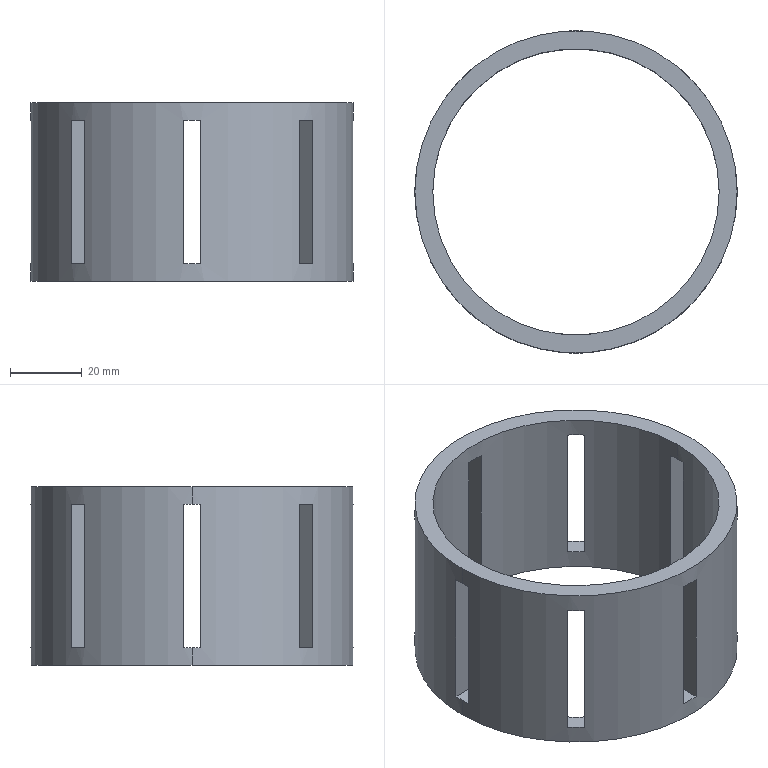Part | SolidWorks | features CirPattern 1, Cut 1, Extrusion 1 | 1 solid | 38 faces | box 90 x 90 x 50 mm | volume 58754 mm3 | plane 34 | cylinder 4 | commonest cylinder face diameters 80 x2 90 x2
STEP:
#1=CARTESIAN_POINT('',(-597.384,-129.922,45.));
#2=VERTEX_POINT('',#1);
#3=CARTESIAN_POINT('',(-597.384,-129.922,5.));
#4=VERTEX_POINT('',#3);
#5=CARTESIAN_POINT('',(-597.384,-129.922,50.));
#6=DIRECTION('',(0.,0.,-1.));
#7=VECTOR('',#6,1000.);
#8=LINE('',#5,#7);
#9=EDGE_CURVE('',#2,#4,#8,.T.);
#10=ORIENTED_EDGE('',*,*,#9,.F.);
#11=CARTESIAN_POINT('',(-602.384,-129.922,45.));
#12=VERTEX_POINT('',#11);
#13=CARTESIAN_POINT('',(-599.884,-90.,45.));
#14=DIRECTION('',(0.,0.,1.));
#15=DIRECTION('',(1.,0.,0.));
#16=AXIS2_PLACEMENT_3D('',#13,#14,#15);
#17=CIRCLE('',#16,40.);
#18=EDGE_CURVE('',#12,#2,#17,.T.);
#19=ORIENTED_EDGE('',*,*,#18,.F.);
#20=CARTESIAN_POINT('',(-602.384,-129.922,5.));
#21=VERTEX_POINT('',#20);
#22=CARTESIAN_POINT('',(-602.384,-129.922,50.));
#23=DIRECTION('',(0.,0.,1.));
#24=VECTOR('',#23,1000.);
#25=LINE('',#22,#24);
#26=EDGE_CURVE('',#21,#12,#25,.T.);
#27=ORIENTED_EDGE('',*,*,#26,.F.);
#28=CARTESIAN_POINT('',(-599.884,-90.,5.));
#29=DIRECTION('',(0.,0.,-1.));
#30=DIRECTION('',(-1.,0.,0.));
#31=AXIS2_PLACEMENT_3D('',#28,#29,#30);
#32=CIRCLE('',#31,40.);
#33=EDGE_CURVE('',#4,#21,#32,.T.);
#34=ORIENTED_EDGE('',*,*,#33,.F.);
#35=EDGE_LOOP('',(#10,#19,#27,#34));
#36=FACE_BOUND('',#35,.T.);
#37=CARTESIAN_POINT('',(-629.881,-116.461,5.));
#38=VERTEX_POINT('',#37);
#39=CARTESIAN_POINT('',(-629.881,-116.461,45.));
#40=VERTEX_POINT('',#39);
#41=CARTESIAN_POINT('',(-629.881,-116.461,50.));
#42=DIRECTION('',(0.,0.,1.));
#43=VECTOR('',#42,1000.);
#44=LINE('',#41,#43);
#45=EDGE_CURVE('',#38,#40,#44,.T.);
#46=ORIENTED_EDGE('',*,*,#45,.F.);
#47=CARTESIAN_POINT('',(-626.345,-119.997,5.));
#48=VERTEX_POINT('',#47);
#49=CARTESIAN_POINT('',(-599.884,-90.,5.));
#50=DIRECTION('',(0.,0.,-1.));
#51=DIRECTION('',(-1.,0.,0.));
#52=AXIS2_PLACEMENT_3D('',#49,#50,#51);
#53=CIRCLE('',#52,40.);
#54=EDGE_CURVE('',#48,#38,#53,.T.);
#55=ORIENTED_EDGE('',*,*,#54,.F.);
#56=CARTESIAN_POINT('',(-626.345,-119.997,45.));
#57=VERTEX_POINT('',#56);
#58=CARTESIAN_POINT('',(-626.345,-119.997,50.));
#59=DIRECTION('',(0.,0.,-1.));
#60=VECTOR('',#59,1000.);
#61=LINE('',#58,#60);
#62=EDGE_CURVE('',#57,#48,#61,.T.);
#63=ORIENTED_EDGE('',*,*,#62,.F.);
#64=CARTESIAN_POINT('',(-599.884,-90.,45.));
#65=DIRECTION('',(0.,0.,1.));
#66=DIRECTION('',(1.,0.,0.));
#67=AXIS2_PLACEMENT_3D('',#64,#65,#66);
#68=CIRCLE('',#67,40.);
#69=EDGE_CURVE('',#40,#57,#68,.T.);
#70=ORIENTED_EDGE('',*,*,#69,.F.);
#71=EDGE_LOOP('',(#46,#55,#63,#70));
#72=FACE_BOUND('',#71,.T.);
#73=CARTESIAN_POINT('',(-569.887,-116.461,45.));
#74=VERTEX_POINT('',#73);
#75=CARTESIAN_POINT('',(-569.887,-116.461,5.));
#76=VERTEX_POINT('',#75);
#77=CARTESIAN_POINT('',(-569.887,-116.461,50.));
#78=DIRECTION('',(0.,0.,-1.));
#79=VECTOR('',#78,1000.);
#80=LINE('',#77,#79);
#81=EDGE_CURVE('',#74,#76,#80,.T.);
#82=ORIENTED_EDGE('',*,*,#81,.F.);
#83=CARTESIAN_POINT('',(-573.423,-119.997,45.));
#84=VERTEX_POINT('',#83);
#85=CARTESIAN_POINT('',(-599.884,-90.,45.));
#86=DIRECTION('',(0.,0.,1.));
#87=DIRECTION('',(1.,0.,0.));
#88=AXIS2_PLACEMENT_3D('',#85,#86,#87);
#89=CIRCLE('',#88,40.);
#90=EDGE_CURVE('',#84,#74,#89,.T.);
#91=ORIENTED_EDGE('',*,*,#90,.F.);
#92=CARTESIAN_POINT('',(-573.423,-119.997,5.));
#93=VERTEX_POINT('',#92);
#94=CARTESIAN_POINT('',(-573.423,-119.997,50.));
#95=DIRECTION('',(0.,0.,1.));
#96=VECTOR('',#95,1000.);
#97=LINE('',#94,#96);
#98=EDGE_CURVE('',#93,#84,#97,.T.);
#99=ORIENTED_EDGE('',*,*,#98,.F.);
#100=CARTESIAN_POINT('',(-599.884,-90.,5.));
#101=DIRECTION('',(0.,0.,-1.));
#102=DIRECTION('',(-1.,0.,0.));
#103=AXIS2_PLACEMENT_3D('',#100,#101,#102);
#104=CIRCLE('',#103,40.);
#105=EDGE_CURVE('',#76,#93,#104,.T.);
#106=ORIENTED_EDGE('',*,*,#105,.F.);
#107=EDGE_LOOP('',(#82,#91,#99,#106));
#108=FACE_BOUND('',#107,.T.);
#109=CARTESIAN_POINT('',(-639.884,-90.,50.));
#110=VERTEX_POINT('',#109);
#111=CARTESIAN_POINT('',(-559.884,-90.,50.));
#112=VERTEX_POINT('',#111);
#113=CARTESIAN_POINT('',(-599.884,-90.,50.));
#114=DIRECTION('',(0.,0.,1.));
#115=DIRECTION('',(1.,0.,0.));
#116=AXIS2_PLACEMENT_3D('',#113,#114,#115);
#117=CIRCLE('',#116,40.);
#118=EDGE_CURVE('',#110,#112,#117,.T.);
#119=ORIENTED_EDGE('',*,*,#118,.T.);
#120=CARTESIAN_POINT('',(-559.884,-90.,45.));
#121=VERTEX_POINT('',#120);
#122=CARTESIAN_POINT('',(-559.884,-90.,50.));
#123=DIRECTION('',(0.,0.,-1.));
#124=VECTOR('',#123,1000.);
#125=LINE('',#122,#124);
#126=EDGE_CURVE('',#112,#121,#125,.T.);
#127=ORIENTED_EDGE('',*,*,#126,.T.);
#128=CARTESIAN_POINT('',(-559.962,-92.5,45.));
#129=VERTEX_POINT('',#128);
#130=CARTESIAN_POINT('',(-599.884,-90.,45.));
#131=DIRECTION('',(0.,0.,1.));
#132=DIRECTION('',(1.,0.,0.));
#133=AXIS2_PLACEMENT_3D('',#130,#131,#132);
#134=CIRCLE('',#133,40.);
#135=EDGE_CURVE('',#129,#121,#134,.T.);
#136=ORIENTED_EDGE('',*,*,#135,.F.);
#137=CARTESIAN_POINT('',(-559.962,-92.5,5.));
#138=VERTEX_POINT('',#137);
#139=CARTESIAN_POINT('',(-559.962,-92.5,50.));
#140=DIRECTION('',(0.,0.,1.));
#141=VECTOR('',#140,1000.);
#142=LINE('',#139,#141);
#143=EDGE_CURVE('',#138,#129,#142,.T.);
#144=ORIENTED_EDGE('',*,*,#143,.F.);
#145=CARTESIAN_POINT('',(-559.884,-90.,5.));
#146=VERTEX_POINT('',#145);
#147=CARTESIAN_POINT('',(-599.884,-90.,5.));
#148=DIRECTION('',(0.,0.,-1.));
#149=DIRECTION('',(-1.,0.,0.));
#150=AXIS2_PLACEMENT_3D('',#147,#148,#149);
#151=CIRCLE('',#150,40.);
#152=EDGE_CURVE('',#146,#138,#151,.T.);
#153=ORIENTED_EDGE('',*,*,#152,.F.);
#154=CARTESIAN_POINT('',(-559.884,-90.,0.));
#155=VERTEX_POINT('',#154);
#156=CARTESIAN_POINT('',(-559.884,-90.,50.));
#157=DIRECTION('',(0.,0.,-1.));
#158=VECTOR('',#157,1000.);
#159=LINE('',#156,#158);
#160=EDGE_CURVE('',#146,#155,#159,.T.);
#161=ORIENTED_EDGE('',*,*,#160,.T.);
#162=CARTESIAN_POINT('',(-639.884,-90.,0.));
#163=VERTEX_POINT('',#162);
#164=CARTESIAN_POINT('',(-599.884,-90.,0.));
#165=DIRECTION('',(0.,0.,1.));
#166=DIRECTION('',(1.,0.,0.));
#167=AXIS2_PLACEMENT_3D('',#164,#165,#166);
#168=CIRCLE('',#167,40.);
#169=EDGE_CURVE('',#163,#155,#168,.T.);
#170=ORIENTED_EDGE('',*,*,#169,.F.);
#171=CARTESIAN_POINT('',(-639.884,-90.,5.));
#172=VERTEX_POINT('',#171);
#173=CARTESIAN_POINT('',(-639.884,-90.,50.));
#174=DIRECTION('',(0.,0.,-1.));
#175=VECTOR('',#174,1000.);
#176=LINE('',#173,#175);
#177=EDGE_CURVE('',#172,#163,#176,.T.);
#178=ORIENTED_EDGE('',*,*,#177,.F.);
#179=CARTESIAN_POINT('',(-639.806,-92.5,5.));
#180=VERTEX_POINT('',#179);
#181=CARTESIAN_POINT('',(-599.884,-90.,5.));
#182=DIRECTION('',(0.,0.,-1.));
#183=DIRECTION('',(-1.,0.,0.));
#184=AXIS2_PLACEMENT_3D('',#181,#182,#183);
#185=CIRCLE('',#184,40.);
#186=EDGE_CURVE('',#180,#172,#185,.T.);
#187=ORIENTED_EDGE('',*,*,#186,.F.);
#188=CARTESIAN_POINT('',(-639.806,-92.5,45.));
#189=VERTEX_POINT('',#188);
#190=CARTESIAN_POINT('',(-639.806,-92.5,50.));
#191=DIRECTION('',(0.,0.,-1.));
#192=VECTOR('',#191,1000.);
#193=LINE('',#190,#192);
#194=EDGE_CURVE('',#189,#180,#193,.T.);
#195=ORIENTED_EDGE('',*,*,#194,.F.);
#196=CARTESIAN_POINT('',(-639.884,-90.,45.));
#197=VERTEX_POINT('',#196);
#198=CARTESIAN_POINT('',(-599.884,-90.,45.));
#199=DIRECTION('',(0.,0.,1.));
#200=DIRECTION('',(1.,0.,0.));
#201=AXIS2_PLACEMENT_3D('',#198,#199,#200);
#202=CIRCLE('',#201,40.);
#203=EDGE_CURVE('',#197,#189,#202,.T.);
#204=ORIENTED_EDGE('',*,*,#203,.F.);
#205=CARTESIAN_POINT('',(-639.884,-90.,50.));
#206=DIRECTION('',(0.,0.,-1.));
#207=VECTOR('',#206,1000.);
#208=LINE('',#205,#207);
#209=EDGE_CURVE('',#110,#197,#208,.T.);
#210=ORIENTED_EDGE('',*,*,#209,.F.);
#211=EDGE_LOOP('',(#119,#127,#136,#144,#153,#161,#170,#178,#187,#195,#204,#210));
#212=FACE_OUTER_BOUND('',#211,.T.);
#213=CARTESIAN_POINT('',(-599.884,-90.,50.));
#214=DIRECTION('',(0.,0.,-1.));
#215=DIRECTION('',(-1.,0.,0.));
#216=AXIS2_PLACEMENT_3D('',#213,#214,#215);
#217=CYLINDRICAL_SURFACE('',#216,40.);
#218=ADVANCED_FACE('',(#36,#72,#108,#212),#217,.F.);
#219=CARTESIAN_POINT('',(-602.384,-45.069,5.));
#220=VERTEX_POINT('',#219);
#221=CARTESIAN_POINT('',(-597.384,-45.069,5.));
#222=VERTEX_POINT('',#221);
#223=CARTESIAN_POINT('',(-599.884,-90.,5.));
#224=DIRECTION('',(0.,0.,-1.));
#225=DIRECTION('',(-1.,0.,0.));
#226=AXIS2_PLACEMENT_3D('',#223,#224,#225);
#227=CIRCLE('',#226,45.);
#228=EDGE_CURVE('',#220,#222,#227,.T.);
#229=ORIENTED_EDGE('',*,*,#228,.T.);
#230=CARTESIAN_POINT('',(-597.384,-45.069,45.));
#231=VERTEX_POINT('',#230);
#232=CARTESIAN_POINT('',(-597.384,-45.069,50.));
#233=DIRECTION('',(0.,0.,1.));
#234=VECTOR('',#233,1000.);
#235=LINE('',#232,#234);
#236=EDGE_CURVE('',#222,#231,#235,.T.);
#237=ORIENTED_EDGE('',*,*,#236,.T.);
#238=CARTESIAN_POINT('',(-602.384,-45.069,45.));
#239=VERTEX_POINT('',#238);
#240=CARTESIAN_POINT('',(-599.884,-90.,45.));
#241=DIRECTION('',(0.,0.,1.));
#242=DIRECTION('',(1.,0.,0.));
#243=AXIS2_PLACEMENT_3D('',#240,#241,#242);
#244=CIRCLE('',#243,45.);
#245=EDGE_CURVE('',#231,#239,#244,.T.);
#246=ORIENTED_EDGE('',*,*,#245,.T.);
#247=CARTESIAN_POINT('',(-602.384,-45.069,50.));
#248=DIRECTION('',(0.,0.,-1.));
#249=VECTOR('',#248,1000.);
#250=LINE('',#247,#249);
#251=EDGE_CURVE('',#239,#220,#250,.T.);
#252=ORIENTED_EDGE('',*,*,#251,.T.);
#253=EDGE_LOOP('',(#229,#237,#246,#252));
#254=FACE_BOUND('',#253,.T.);
#255=CARTESIAN_POINT('',(-566.346,-59.997,45.));
#256=VERTEX_POINT('',#255);
#257=CARTESIAN_POINT('',(-569.881,-56.462,45.));
#258=VERTEX_POINT('',#257);
#259=CARTESIAN_POINT('',(-599.884,-90.,45.));
#260=DIRECTION('',(0.,0.,1.));
#261=DIRECTION('',(1.,0.,0.));
#262=AXIS2_PLACEMENT_3D('',#259,#260,#261);
#263=CIRCLE('',#262,45.);
#264=EDGE_CURVE('',#256,#258,#263,.T.);
#265=ORIENTED_EDGE('',*,*,#264,.T.);
#266=CARTESIAN_POINT('',(-569.881,-56.462,5.));
#267=VERTEX_POINT('',#266);
#268=CARTESIAN_POINT('',(-569.881,-56.462,50.));
#269=DIRECTION('',(0.,0.,-1.));
#270=VECTOR('',#269,1000.);
#271=LINE('',#268,#270);
#272=EDGE_CURVE('',#258,#267,#271,.T.);
#273=ORIENTED_EDGE('',*,*,#272,.T.);
#274=CARTESIAN_POINT('',(-566.346,-59.997,5.));
#275=VERTEX_POINT('',#274);
#276=CARTESIAN_POINT('',(-599.884,-90.,5.));
#277=DIRECTION('',(0.,0.,-1.));
#278=DIRECTION('',(-1.,0.,0.));
#279=AXIS2_PLACEMENT_3D('',#276,#277,#278);
#280=CIRCLE('',#279,45.);
#281=EDGE_CURVE('',#267,#275,#280,.T.);
#282=ORIENTED_EDGE('',*,*,#281,.T.);
#283=CARTESIAN_POINT('',(-566.346,-59.997,50.));
#284=DIRECTION('',(0.,0.,1.));
#285=VECTOR('',#284,1000.);
#286=LINE('',#283,#285);
#287=EDGE_CURVE('',#275,#256,#286,.T.);
#288=ORIENTED_EDGE('',*,*,#287,.T.);
#289=EDGE_LOOP('',(#265,#273,#282,#288));
#290=FACE_BOUND('',#289,.T.);
#291=CARTESIAN_POINT('',(-629.887,-56.462,5.));
#292=VERTEX_POINT('',#291);
#293=CARTESIAN_POINT('',(-629.887,-56.462,45.));
#294=VERTEX_POINT('',#293);
#295=CARTESIAN_POINT('',(-629.887,-56.462,50.));
#296=DIRECTION('',(0.,0.,1.));
#297=VECTOR('',#296,1000.);
#298=LINE('',#295,#297);
#299=EDGE_CURVE('',#292,#294,#298,.T.);
#300=ORIENTED_EDGE('',*,*,#299,.T.);
#301=CARTESIAN_POINT('',(-633.423,-59.997,45.));
#302=VERTEX_POINT('',#301);
#303=CARTESIAN_POINT('',(-599.884,-90.,45.));
#304=DIRECTION('',(0.,0.,1.));
#305=DIRECTION('',(1.,0.,0.));
#306=AXIS2_PLACEMENT_3D('',#303,#304,#305);
#307=CIRCLE('',#306,45.);
#308=EDGE_CURVE('',#294,#302,#307,.T.);
#309=ORIENTED_EDGE('',*,*,#308,.T.);
#310=CARTESIAN_POINT('',(-633.423,-59.997,5.));
#311=VERTEX_POINT('',#310);
#312=CARTESIAN_POINT('',(-633.423,-59.997,50.));
#313=DIRECTION('',(0.,0.,-1.));
#314=VECTOR('',#313,1000.);
#315=LINE('',#312,#314);
#316=EDGE_CURVE('',#302,#311,#315,.T.);
#317=ORIENTED_EDGE('',*,*,#316,.T.);
#318=CARTESIAN_POINT('',(-599.884,-90.,5.));
#319=DIRECTION('',(0.,0.,-1.));
#320=DIRECTION('',(-1.,0.,0.));
#321=AXIS2_PLACEMENT_3D('',#318,#319,#320);
#322=CIRCLE('',#321,45.);
#323=EDGE_CURVE('',#311,#292,#322,.T.);
#324=ORIENTED_EDGE('',*,*,#323,.T.);
#325=EDGE_LOOP('',(#300,#309,#317,#324));
#326=FACE_BOUND('',#325,.T.);
#327=CARTESIAN_POINT('',(-554.884,-90.,50.));
#328=VERTEX_POINT('',#327);
#329=CARTESIAN_POINT('',(-644.884,-90.,50.));
#330=VERTEX_POINT('',#329);
#331=CARTESIAN_POINT('',(-599.884,-90.,50.));
#332=DIRECTION('',(0.,0.,1.));
#333=DIRECTION('',(1.,0.,0.));
#334=AXIS2_PLACEMENT_3D('',#331,#332,#333);
#335=CIRCLE('',#334,45.);
#336=EDGE_CURVE('',#328,#330,#335,.T.);
#337=ORIENTED_EDGE('',*,*,#336,.F.);
#338=CARTESIAN_POINT('',(-554.884,-90.,45.));
#339=VERTEX_POINT('',#338);
#340=CARTESIAN_POINT('',(-554.884,-90.,50.));
#341=DIRECTION('',(0.,0.,-1.));
#342=VECTOR('',#341,1000.);
#343=LINE('',#340,#342);
#344=EDGE_CURVE('',#328,#339,#343,.T.);
#345=ORIENTED_EDGE('',*,*,#344,.T.);
#346=CARTESIAN_POINT('',(-554.954,-87.5,45.));
#347=VERTEX_POINT('',#346);
#348=CARTESIAN_POINT('',(-599.884,-90.,45.));
#349=DIRECTION('',(0.,0.,1.));
#350=DIRECTION('',(1.,0.,0.));
#351=AXIS2_PLACEMENT_3D('',#348,#349,#350);
#352=CIRCLE('',#351,45.);
#353=EDGE_CURVE('',#339,#347,#352,.T.);
#354=ORIENTED_EDGE('',*,*,#353,.T.);
#355=CARTESIAN_POINT('',(-554.954,-87.5,5.));
#356=VERTEX_POINT('',#355);
#357=CARTESIAN_POINT('',(-554.954,-87.5,50.));
#358=DIRECTION('',(0.,0.,-1.));
#359=VECTOR('',#358,1000.);
#360=LINE('',#357,#359);
#361=EDGE_CURVE('',#347,#356,#360,.T.);
#362=ORIENTED_EDGE('',*,*,#361,.T.);
#363=CARTESIAN_POINT('',(-554.884,-90.,5.));
#364=VERTEX_POINT('',#363);
#365=CARTESIAN_POINT('',(-599.884,-90.,5.));
#366=DIRECTION('',(0.,0.,-1.));
#367=DIRECTION('',(-1.,0.,0.));
#368=AXIS2_PLACEMENT_3D('',#365,#366,#367);
#369=CIRCLE('',#368,45.);
#370=EDGE_CURVE('',#356,#364,#369,.T.);
#371=ORIENTED_EDGE('',*,*,#370,.T.);
#372=CARTESIAN_POINT('',(-554.884,-90.,0.));
#373=VERTEX_POINT('',#372);
#374=CARTESIAN_POINT('',(-554.884,-90.,50.));
#375=DIRECTION('',(0.,0.,-1.));
#376=VECTOR('',#375,1000.);
#377=LINE('',#374,#376);
#378=EDGE_CURVE('',#364,#373,#377,.T.);
#379=ORIENTED_EDGE('',*,*,#378,.T.);
#380=CARTESIAN_POINT('',(-644.884,-90.,0.));
#381=VERTEX_POINT('',#380);
#382=CARTESIAN_POINT('',(-599.884,-90.,0.));
#383=DIRECTION('',(0.,0.,1.));
#384=DIRECTION('',(1.,0.,0.));
#385=AXIS2_PLACEMENT_3D('',#382,#383,#384);
#386=CIRCLE('',#385,45.);
#387=EDGE_CURVE('',#373,#381,#386,.T.);
#388=ORIENTED_EDGE('',*,*,#387,.T.);
#389=CARTESIAN_POINT('',(-644.884,-90.,5.));
#390=VERTEX_POINT('',#389);
#391=CARTESIAN_POINT('',(-644.884,-90.,50.));
#392=DIRECTION('',(0.,0.,-1.));
#393=VECTOR('',#392,1000.);
#394=LINE('',#391,#393);
#395=EDGE_CURVE('',#390,#381,#394,.T.);
#396=ORIENTED_EDGE('',*,*,#395,.F.);
#397=CARTESIAN_POINT('',(-644.815,-87.5,5.));
#398=VERTEX_POINT('',#397);
#399=CARTESIAN_POINT('',(-599.884,-90.,5.));
#400=DIRECTION('',(0.,0.,-1.));
#401=DIRECTION('',(-1.,0.,0.));
#402=AXIS2_PLACEMENT_3D('',#399,#400,#401);
#403=CIRCLE('',#402,45.);
#404=EDGE_CURVE('',#390,#398,#403,.T.);
#405=ORIENTED_EDGE('',*,*,#404,.T.);
#406=CARTESIAN_POINT('',(-644.815,-87.5,45.));
#407=VERTEX_POINT('',#406);
#408=CARTESIAN_POINT('',(-644.815,-87.5,50.));
#409=DIRECTION('',(0.,0.,1.));
#410=VECTOR('',#409,1000.);
#411=LINE('',#408,#410);
#412=EDGE_CURVE('',#398,#407,#411,.T.);
#413=ORIENTED_EDGE('',*,*,#412,.T.);
#414=CARTESIAN_POINT('',(-644.884,-90.,45.));
#415=VERTEX_POINT('',#414);
#416=CARTESIAN_POINT('',(-599.884,-90.,45.));
#417=DIRECTION('',(0.,0.,1.));
#418=DIRECTION('',(1.,0.,0.));
#419=AXIS2_PLACEMENT_3D('',#416,#417,#418);
#420=CIRCLE('',#419,45.);
#421=EDGE_CURVE('',#407,#415,#420,.T.);
#422=ORIENTED_EDGE('',*,*,#421,.T.);
#423=CARTESIAN_POINT('',(-644.884,-90.,50.));
#424=DIRECTION('',(0.,0.,-1.));
#425=VECTOR('',#424,1000.);
#426=LINE('',#423,#425);
#427=EDGE_CURVE('',#330,#415,#426,.T.);
#428=ORIENTED_EDGE('',*,*,#427,.F.);
#429=EDGE_LOOP('',(#337,#345,#354,#362,#371,#379,#388,#396,#405,#413,#422,#428));
#430=FACE_OUTER_BOUND('',#429,.T.);
#431=CARTESIAN_POINT('',(-599.884,-90.,50.));
#432=DIRECTION('',(0.,0.,-1.));
#433=DIRECTION('',(-1.,0.,0.));
#434=AXIS2_PLACEMENT_3D('',#431,#432,#433);
#435=CYLINDRICAL_SURFACE('',#434,45.);
#436=ADVANCED_FACE('',(#254,#290,#326,#430),#435,.T.);
#437=CARTESIAN_POINT('',(-599.884,-90.,50.));
#438=DIRECTION('',(0.,0.,1.));
#439=DIRECTION('',(1.,0.,0.));
#440=AXIS2_PLACEMENT_3D('',#437,#438,#439);
#441=CIRCLE('',#440,45.);
#442=EDGE_CURVE('',#330,#328,#441,.T.);
#443=ORIENTED_EDGE('',*,*,#442,.T.);
#444=ORIENTED_EDGE('',*,*,#336,.T.);
#445=EDGE_LOOP('',(#443,#444));
#446=FACE_OUTER_BOUND('',#445,.T.);
#447=ORIENTED_EDGE('',*,*,#118,.F.);
#448=CARTESIAN_POINT('',(-599.884,-90.,50.));
#449=DIRECTION('',(0.,0.,1.));
#450=DIRECTION('',(1.,0.,0.));
#451=AXIS2_PLACEMENT_3D('',#448,#449,#450);
#452=CIRCLE('',#451,40.);
#453=EDGE_CURVE('',#112,#110,#452,.T.);
#454=ORIENTED_EDGE('',*,*,#453,.F.);
#455=EDGE_LOOP('',(#447,#454));
#456=FACE_BOUND('',#455,.T.);
#457=CARTESIAN_POINT('',(-599.884,-90.,50.));
#458=DIRECTION('',(0.,0.,1.));
#459=DIRECTION('',(1.,0.,0.));
#460=AXIS2_PLACEMENT_3D('',#457,#458,#459);
#461=PLANE('',#460);
#462=ADVANCED_FACE('',(#446,#456),#461,.T.);
#463=CARTESIAN_POINT('',(-599.884,-90.,0.));
#464=DIRECTION('',(0.,0.,1.));
#465=DIRECTION('',(1.,0.,0.));
#466=AXIS2_PLACEMENT_3D('',#463,#464,#465);
#467=CIRCLE('',#466,45.);
#468=EDGE_CURVE('',#381,#373,#467,.T.);
#469=ORIENTED_EDGE('',*,*,#468,.F.);
#470=ORIENTED_EDGE('',*,*,#387,.F.);
#471=EDGE_LOOP('',(#469,#470));
#472=FACE_OUTER_BOUND('',#471,.T.);
#473=ORIENTED_EDGE('',*,*,#169,.T.);
#474=CARTESIAN_POINT('',(-599.884,-90.,0.));
#475=DIRECTION('',(0.,0.,1.));
#476=DIRECTION('',(1.,0.,0.));
#477=AXIS2_PLACEMENT_3D('',#474,#475,#476);
#478=CIRCLE('',#477,40.);
#479=EDGE_CURVE('',#155,#163,#478,.T.);
#480=ORIENTED_EDGE('',*,*,#479,.T.);
#481=EDGE_LOOP('',(#473,#480));
#482=FACE_BOUND('',#481,.T.);
#483=CARTESIAN_POINT('',(-599.884,-90.,0.));
#484=DIRECTION('',(0.,0.,1.));
#485=DIRECTION('',(1.,0.,0.));
#486=AXIS2_PLACEMENT_3D('',#483,#484,#485);
#487=PLANE('',#486);
#488=ADVANCED_FACE('',(#472,#482),#487,.F.);
#489=ORIENTED_EDGE('',*,*,#344,.F.);
#490=ORIENTED_EDGE('',*,*,#442,.F.);
#491=ORIENTED_EDGE('',*,*,#427,.T.);
#492=CARTESIAN_POINT('',(-644.815,-92.5,45.));
#493=VERTEX_POINT('',#492);
#494=CARTESIAN_POINT('',(-599.884,-90.,45.));
#495=DIRECTION('',(0.,0.,1.));
#496=DIRECTION('',(1.,0.,0.));
#497=AXIS2_PLACEMENT_3D('',#494,#495,#496);
#498=CIRCLE('',#497,45.);
#499=EDGE_CURVE('',#415,#493,#498,.T.);
#500=ORIENTED_EDGE('',*,*,#499,.T.);
#501=CARTESIAN_POINT('',(-644.815,-92.5,5.));
#502=VERTEX_POINT('',#501);
#503=CARTESIAN_POINT('',(-644.815,-92.5,50.));
#504=DIRECTION('',(0.,0.,-1.));
#505=VECTOR('',#504,1000.);
#506=LINE('',#503,#505);
#507=EDGE_CURVE('',#493,#502,#506,.T.);
#508=ORIENTED_EDGE('',*,*,#507,.T.);
#509=CARTESIAN_POINT('',(-599.884,-90.,5.));
#510=DIRECTION('',(0.,0.,-1.));
#511=DIRECTION('',(-1.,0.,0.));
#512=AXIS2_PLACEMENT_3D('',#509,#510,#511);
#513=CIRCLE('',#512,45.);
#514=EDGE_CURVE('',#502,#390,#513,.T.);
#515=ORIENTED_EDGE('',*,*,#514,.T.);
#516=ORIENTED_EDGE('',*,*,#395,.T.);
#517=ORIENTED_EDGE('',*,*,#468,.T.);
#518=ORIENTED_EDGE('',*,*,#378,.F.);
#519=CARTESIAN_POINT('',(-554.954,-92.5,5.));
#520=VERTEX_POINT('',#519);
#521=CARTESIAN_POINT('',(-599.884,-90.,5.));
#522=DIRECTION('',(0.,0.,-1.));
#523=DIRECTION('',(-1.,0.,0.));
#524=AXIS2_PLACEMENT_3D('',#521,#522,#523);
#525=CIRCLE('',#524,45.);
#526=EDGE_CURVE('',#364,#520,#525,.T.);
#527=ORIENTED_EDGE('',*,*,#526,.T.);
#528=CARTESIAN_POINT('',(-554.954,-92.5,45.));
#529=VERTEX_POINT('',#528);
#530=CARTESIAN_POINT('',(-554.954,-92.5,50.));
#531=DIRECTION('',(0.,0.,1.));
#532=VECTOR('',#531,1000.);
#533=LINE('',#530,#532);
#534=EDGE_CURVE('',#520,#529,#533,.T.);
#535=ORIENTED_EDGE('',*,*,#534,.T.);
#536=CARTESIAN_POINT('',(-599.884,-90.,45.));
#537=DIRECTION('',(0.,0.,1.));
#538=DIRECTION('',(1.,0.,0.));
#539=AXIS2_PLACEMENT_3D('',#536,#537,#538);
#540=CIRCLE('',#539,45.);
#541=EDGE_CURVE('',#529,#339,#540,.T.);
#542=ORIENTED_EDGE('',*,*,#541,.T.);
#543=EDGE_LOOP('',(#489,#490,#491,#500,#508,#515,#516,#517,#518,#527,#535,#542));
#544=FACE_OUTER_BOUND('',#543,.T.);
#545=CARTESIAN_POINT('',(-569.881,-123.538,45.));
#546=VERTEX_POINT('',#545);
#547=CARTESIAN_POINT('',(-566.346,-120.003,45.));
#548=VERTEX_POINT('',#547);
#549=CARTESIAN_POINT('',(-599.884,-90.,45.));
#550=DIRECTION('',(0.,0.,1.));
#551=DIRECTION('',(1.,0.,0.));
#552=AXIS2_PLACEMENT_3D('',#549,#550,#551);
#553=CIRCLE('',#552,45.);
#554=EDGE_CURVE('',#546,#548,#553,.T.);
#555=ORIENTED_EDGE('',*,*,#554,.T.);
#556=CARTESIAN_POINT('',(-566.346,-120.003,5.));
#557=VERTEX_POINT('',#556);
#558=CARTESIAN_POINT('',(-566.346,-120.003,50.));
#559=DIRECTION('',(0.,0.,-1.));
#560=VECTOR('',#559,1000.);
#561=LINE('',#558,#560);
#562=EDGE_CURVE('',#548,#557,#561,.T.);
#563=ORIENTED_EDGE('',*,*,#562,.T.);
#564=CARTESIAN_POINT('',(-569.881,-123.538,5.));
#565=VERTEX_POINT('',#564);
#566=CARTESIAN_POINT('',(-599.884,-90.,5.));
#567=DIRECTION('',(0.,0.,-1.));
#568=DIRECTION('',(-1.,0.,0.));
#569=AXIS2_PLACEMENT_3D('',#566,#567,#568);
#570=CIRCLE('',#569,45.);
#571=EDGE_CURVE('',#557,#565,#570,.T.);
#572=ORIENTED_EDGE('',*,*,#571,.T.);
#573=CARTESIAN_POINT('',(-569.881,-123.538,50.));
#574=DIRECTION('',(0.,0.,1.));
#575=VECTOR('',#574,1000.);
#576=LINE('',#573,#575);
#577=EDGE_CURVE('',#565,#546,#576,.T.);
#578=ORIENTED_EDGE('',*,*,#577,.T.);
#579=EDGE_LOOP('',(#555,#563,#572,#578));
#580=FACE_BOUND('',#579,.T.);
#581=CARTESIAN_POINT('',(-629.887,-123.538,5.));
#582=VERTEX_POINT('',#581);
#583=CARTESIAN_POINT('',(-633.423,-120.003,5.));
#584=VERTEX_POINT('',#583);
#585=CARTESIAN_POINT('',(-599.884,-90.,5.));
#586=DIRECTION('',(0.,0.,-1.));
#587=DIRECTION('',(-1.,0.,0.));
#588=AXIS2_PLACEMENT_3D('',#585,#586,#587);
#589=CIRCLE('',#588,45.);
#590=EDGE_CURVE('',#582,#584,#589,.T.);
#591=ORIENTED_EDGE('',*,*,#590,.T.);
#592=CARTESIAN_POINT('',(-633.423,-120.003,45.));
#593=VERTEX_POINT('',#592);
#594=CARTESIAN_POINT('',(-633.423,-120.003,50.));
#595=DIRECTION('',(0.,0.,1.));
#596=VECTOR('',#595,1000.);
#597=LINE('',#594,#596);
#598=EDGE_CURVE('',#584,#593,#597,.T.);
#599=ORIENTED_EDGE('',*,*,#598,.T.);
#600=CARTESIAN_POINT('',(-629.887,-123.538,45.));
#601=VERTEX_POINT('',#600);
#602=CARTESIAN_POINT('',(-599.884,-90.,45.));
#603=DIRECTION('',(0.,0.,1.));
#604=DIRECTION('',(1.,0.,0.));
#605=AXIS2_PLACEMENT_3D('',#602,#603,#604);
#606=CIRCLE('',#605,45.);
#607=EDGE_CURVE('',#593,#601,#606,.T.);
#608=ORIENTED_EDGE('',*,*,#607,.T.);
#609=CARTESIAN_POINT('',(-629.887,-123.538,50.));
#610=DIRECTION('',(0.,0.,-1.));
#611=VECTOR('',#610,1000.);
#612=LINE('',#609,#611);
#613=EDGE_CURVE('',#601,#582,#612,.T.);
#614=ORIENTED_EDGE('',*,*,#613,.T.);
#615=EDGE_LOOP('',(#591,#599,#608,#614));
#616=FACE_BOUND('',#615,.T.);
#617=CARTESIAN_POINT('',(-597.384,-134.931,45.));
#618=VERTEX_POINT('',#617);
#619=CARTESIAN_POINT('',(-597.384,-134.931,5.));
#620=VERTEX_POINT('',#619);
#621=CARTESIAN_POINT('',(-597.384,-134.931,50.));
#622=DIRECTION('',(0.,0.,-1.));
#623=VECTOR('',#622,1000.);
#624=LINE('',#621,#623);
#625=EDGE_CURVE('',#618,#620,#624,.T.);
#626=ORIENTED_EDGE('',*,*,#625,.T.);
#627=CARTESIAN_POINT('',(-602.384,-134.931,5.));
#628=VERTEX_POINT('',#627);
#629=CARTESIAN_POINT('',(-599.884,-90.,5.));
#630=DIRECTION('',(0.,0.,-1.));
#631=DIRECTION('',(-1.,0.,0.));
#632=AXIS2_PLACEMENT_3D('',#629,#630,#631);
#633=CIRCLE('',#632,45.);
#634=EDGE_CURVE('',#620,#628,#633,.T.);
#635=ORIENTED_EDGE('',*,*,#634,.T.);
#636=CARTESIAN_POINT('',(-602.384,-134.931,45.));
#637=VERTEX_POINT('',#636);
#638=CARTESIAN_POINT('',(-602.384,-134.931,50.));
#639=DIRECTION('',(0.,0.,1.));
#640=VECTOR('',#639,1000.);
#641=LINE('',#638,#640);
#642=EDGE_CURVE('',#628,#637,#641,.T.);
#643=ORIENTED_EDGE('',*,*,#642,.T.);
#644=CARTESIAN_POINT('',(-599.884,-90.,45.));
#645=DIRECTION('',(0.,0.,1.));
#646=DIRECTION('',(1.,0.,0.));
#647=AXIS2_PLACEMENT_3D('',#644,#645,#646);
#648=CIRCLE('',#647,45.);
#649=EDGE_CURVE('',#637,#618,#648,.T.);
#650=ORIENTED_EDGE('',*,*,#649,.T.);
#651=EDGE_LOOP('',(#626,#635,#643,#650));
#652=FACE_BOUND('',#651,.T.);
#653=CARTESIAN_POINT('',(-599.884,-90.,50.));
#654=DIRECTION('',(0.,0.,-1.));
#655=DIRECTION('',(-1.,0.,0.));
#656=AXIS2_PLACEMENT_3D('',#653,#654,#655);
#657=CYLINDRICAL_SURFACE('',#656,45.);
#658=ADVANCED_FACE('',(#544,#580,#616,#652),#657,.T.);
#659=ORIENTED_EDGE('',*,*,#126,.F.);
#660=ORIENTED_EDGE('',*,*,#453,.T.);
#661=ORIENTED_EDGE('',*,*,#209,.T.);
#662=CARTESIAN_POINT('',(-639.806,-87.5,45.));
#663=VERTEX_POINT('',#662);
#664=CARTESIAN_POINT('',(-599.884,-90.,45.));
#665=DIRECTION('',(0.,0.,1.));
#666=DIRECTION('',(1.,0.,0.));
#667=AXIS2_PLACEMENT_3D('',#664,#665,#666);
#668=CIRCLE('',#667,40.);
#669=EDGE_CURVE('',#663,#197,#668,.T.);
#670=ORIENTED_EDGE('',*,*,#669,.F.);
#671=CARTESIAN_POINT('',(-639.806,-87.5,5.));
#672=VERTEX_POINT('',#671);
#673=CARTESIAN_POINT('',(-639.806,-87.5,50.));
#674=DIRECTION('',(0.,0.,1.));
#675=VECTOR('',#674,1000.);
#676=LINE('',#673,#675);
#677=EDGE_CURVE('',#672,#663,#676,.T.);
#678=ORIENTED_EDGE('',*,*,#677,.F.);
#679=CARTESIAN_POINT('',(-599.884,-90.,5.));
#680=DIRECTION('',(0.,0.,-1.));
#681=DIRECTION('',(-1.,0.,0.));
#682=AXIS2_PLACEMENT_3D('',#679,#680,#681);
#683=CIRCLE('',#682,40.);
#684=EDGE_CURVE('',#172,#672,#683,.T.);
#685=ORIENTED_EDGE('',*,*,#684,.F.);
#686=ORIENTED_EDGE('',*,*,#177,.T.);
#687=ORIENTED_EDGE('',*,*,#479,.F.);
#688=ORIENTED_EDGE('',*,*,#160,.F.);
#689=CARTESIAN_POINT('',(-559.962,-87.5,5.));
#690=VERTEX_POINT('',#689);
#691=CARTESIAN_POINT('',(-599.884,-90.,5.));
#692=DIRECTION('',(0.,0.,-1.));
#693=DIRECTION('',(-1.,0.,0.));
#694=AXIS2_PLACEMENT_3D('',#691,#692,#693);
#695=CIRCLE('',#694,40.);
#696=EDGE_CURVE('',#690,#146,#695,.T.);
#697=ORIENTED_EDGE('',*,*,#696,.F.);
#698=CARTESIAN_POINT('',(-559.962,-87.5,45.));
#699=VERTEX_POINT('',#698);
#700=CARTESIAN_POINT('',(-559.962,-87.5,50.));
#701=DIRECTION('',(0.,0.,-1.));
#702=VECTOR('',#701,1000.);
#703=LINE('',#700,#702);
#704=EDGE_CURVE('',#699,#690,#703,.T.);
#705=ORIENTED_EDGE('',*,*,#704,.F.);
#706=CARTESIAN_POINT('',(-599.884,-90.,45.));
#707=DIRECTION('',(0.,0.,1.));
#708=DIRECTION('',(1.,0.,0.));
#709=AXIS2_PLACEMENT_3D('',#706,#707,#708);
#710=CIRCLE('',#709,40.);
#711=EDGE_CURVE('',#121,#699,#710,.T.);
#712=ORIENTED_EDGE('',*,*,#711,.F.);
#713=EDGE_LOOP('',(#659,#660,#661,#670,#678,#685,#686,#687,#688,#697,#705,#712));
#714=FACE_OUTER_BOUND('',#713,.T.);
#715=CARTESIAN_POINT('',(-626.345,-60.003,45.));
#716=VERTEX_POINT('',#715);
#717=CARTESIAN_POINT('',(-629.881,-63.539,45.));
#718=VERTEX_POINT('',#717);
#719=CARTESIAN_POINT('',(-599.884,-90.,45.));
#720=DIRECTION('',(0.,0.,1.));
#721=DIRECTION('',(1.,0.,0.));
#722=AXIS2_PLACEMENT_3D('',#719,#720,#721);
#723=CIRCLE('',#722,40.);
#724=EDGE_CURVE('',#716,#718,#723,.T.);
#725=ORIENTED_EDGE('',*,*,#724,.F.);
#726=CARTESIAN_POINT('',(-626.345,-60.003,5.));
#727=VERTEX_POINT('',#726);
#728=CARTESIAN_POINT('',(-626.345,-60.003,50.));
#729=DIRECTION('',(0.,0.,1.));
#730=VECTOR('',#729,1000.);
#731=LINE('',#728,#730);
#732=EDGE_CURVE('',#727,#716,#731,.T.);
#733=ORIENTED_EDGE('',*,*,#732,.F.);
#734=CARTESIAN_POINT('',(-629.881,-63.539,5.));
#735=VERTEX_POINT('',#734);
#736=CARTESIAN_POINT('',(-599.884,-90.,5.));
#737=DIRECTION('',(0.,0.,-1.));
#738=DIRECTION('',(-1.,0.,0.));
#739=AXIS2_PLACEMENT_3D('',#736,#737,#738);
#740=CIRCLE('',#739,40.);
#741=EDGE_CURVE('',#735,#727,#740,.T.);
#742=ORIENTED_EDGE('',*,*,#741,.F.);
#743=CARTESIAN_POINT('',(-629.881,-63.539,50.));
#744=DIRECTION('',(0.,0.,-1.));
#745=VECTOR('',#744,1000.);
#746=LINE('',#743,#745);
#747=EDGE_CURVE('',#718,#735,#746,.T.);
#748=ORIENTED_EDGE('',*,*,#747,.F.);
#749=EDGE_LOOP('',(#725,#733,#742,#748));
#750=FACE_BOUND('',#749,.T.);
#751=CARTESIAN_POINT('',(-573.423,-60.003,45.));
#752=VERTEX_POINT('',#751);
#753=CARTESIAN_POINT('',(-573.423,-60.003,5.));
#754=VERTEX_POINT('',#753);
#755=CARTESIAN_POINT('',(-573.423,-60.003,50.));
#756=DIRECTION('',(0.,0.,-1.));
#757=VECTOR('',#756,1000.);
#758=LINE('',#755,#757);
#759=EDGE_CURVE('',#752,#754,#758,.T.);
#760=ORIENTED_EDGE('',*,*,#759,.F.);
#761=CARTESIAN_POINT('',(-569.887,-63.539,45.));
#762=VERTEX_POINT('',#761);
#763=CARTESIAN_POINT('',(-599.884,-90.,45.));
#764=DIRECTION('',(0.,0.,1.));
#765=DIRECTION('',(1.,0.,0.));
#766=AXIS2_PLACEMENT_3D('',#763,#764,#765);
#767=CIRCLE('',#766,40.);
#768=EDGE_CURVE('',#762,#752,#767,.T.);
#769=ORIENTED_EDGE('',*,*,#768,.F.);
#770=CARTESIAN_POINT('',(-569.887,-63.539,5.));
#771=VERTEX_POINT('',#770);
#772=CARTESIAN_POINT('',(-569.887,-63.539,50.));
#773=DIRECTION('',(0.,0.,1.));
#774=VECTOR('',#773,1000.);
#775=LINE('',#772,#774);
#776=EDGE_CURVE('',#771,#762,#775,.T.);
#777=ORIENTED_EDGE('',*,*,#776,.F.);
#778=CARTESIAN_POINT('',(-599.884,-90.,5.));
#779=DIRECTION('',(0.,0.,-1.));
#780=DIRECTION('',(-1.,0.,0.));
#781=AXIS2_PLACEMENT_3D('',#778,#779,#780);
#782=CIRCLE('',#781,40.);
#783=EDGE_CURVE('',#754,#771,#782,.T.);
#784=ORIENTED_EDGE('',*,*,#783,.F.);
#785=EDGE_LOOP('',(#760,#769,#777,#784));
#786=FACE_BOUND('',#785,.T.);
#787=CARTESIAN_POINT('',(-597.384,-50.078,5.));
#788=VERTEX_POINT('',#787);
#789=CARTESIAN_POINT('',(-597.384,-50.078,45.));
#790=VERTEX_POINT('',#789);
#791=CARTESIAN_POINT('',(-597.384,-50.078,50.));
#792=DIRECTION('',(0.,0.,1.));
#793=VECTOR('',#792,1000.);
#794=LINE('',#791,#793);
#795=EDGE_CURVE('',#788,#790,#794,.T.);
#796=ORIENTED_EDGE('',*,*,#795,.F.);
#797=CARTESIAN_POINT('',(-602.384,-50.078,5.));
#798=VERTEX_POINT('',#797);
#799=CARTESIAN_POINT('',(-599.884,-90.,5.));
#800=DIRECTION('',(0.,0.,-1.));
#801=DIRECTION('',(-1.,0.,0.));
#802=AXIS2_PLACEMENT_3D('',#799,#800,#801);
#803=CIRCLE('',#802,40.);
#804=EDGE_CURVE('',#798,#788,#803,.T.);
#805=ORIENTED_EDGE('',*,*,#804,.F.);
#806=CARTESIAN_POINT('',(-602.384,-50.078,45.));
#807=VERTEX_POINT('',#806);
#808=CARTESIAN_POINT('',(-602.384,-50.078,50.));
#809=DIRECTION('',(0.,0.,-1.));
#810=VECTOR('',#809,1000.);
#811=LINE('',#808,#810);
#812=EDGE_CURVE('',#807,#798,#811,.T.);
#813=ORIENTED_EDGE('',*,*,#812,.F.);
#814=CARTESIAN_POINT('',(-599.884,-90.,45.));
#815=DIRECTION('',(0.,0.,1.));
#816=DIRECTION('',(1.,0.,0.));
#817=AXIS2_PLACEMENT_3D('',#814,#815,#816);
#818=CIRCLE('',#817,40.);
#819=EDGE_CURVE('',#790,#807,#818,.T.);
#820=ORIENTED_EDGE('',*,*,#819,.F.);
#821=EDGE_LOOP('',(#796,#805,#813,#820));
#822=FACE_BOUND('',#821,.T.);
#823=CARTESIAN_POINT('',(-599.884,-90.,50.));
#824=DIRECTION('',(0.,0.,-1.));
#825=DIRECTION('',(-1.,0.,0.));
#826=AXIS2_PLACEMENT_3D('',#823,#824,#825);
#827=CYLINDRICAL_SURFACE('',#826,40.);
#828=ADVANCED_FACE('',(#714,#750,#786,#822),#827,.F.);
#829=CARTESIAN_POINT('',(-597.384,-135.,5.));
#830=DIRECTION('',(0.,1.,0.));
#831=VECTOR('',#830,1000.);
#832=LINE('',#829,#831);
#833=EDGE_CURVE('',#620,#4,#832,.T.);
#834=ORIENTED_EDGE('',*,*,#833,.T.);
#835=ORIENTED_EDGE('',*,*,#33,.T.);
#836=CARTESIAN_POINT('',(-602.384,-135.,5.));
#837=DIRECTION('',(0.,1.,0.));
#838=VECTOR('',#837,1000.);
#839=LINE('',#836,#838);
#840=EDGE_CURVE('',#628,#21,#839,.T.);
#841=ORIENTED_EDGE('',*,*,#840,.F.);
#842=ORIENTED_EDGE('',*,*,#634,.F.);
#843=EDGE_LOOP('',(#834,#835,#841,#842));
#844=FACE_OUTER_BOUND('',#843,.T.);
#845=CARTESIAN_POINT('',(-602.384,-135.,5.));
#846=DIRECTION('',(0.,0.,-1.));
#847=DIRECTION('',(-1.,0.,0.));
#848=AXIS2_PLACEMENT_3D('',#845,#846,#847);
#849=PLANE('',#848);
#850=ADVANCED_FACE('',(#844),#849,.F.);
#851=ORIENTED_EDGE('',*,*,#840,.T.);
#852=ORIENTED_EDGE('',*,*,#26,.T.);
#853=CARTESIAN_POINT('',(-602.384,-135.,45.));
#854=DIRECTION('',(0.,1.,0.));
#855=VECTOR('',#854,1000.);
#856=LINE('',#853,#855);
#857=EDGE_CURVE('',#637,#12,#856,.T.);
#858=ORIENTED_EDGE('',*,*,#857,.F.);
#859=ORIENTED_EDGE('',*,*,#642,.F.);
#860=EDGE_LOOP('',(#851,#852,#858,#859));
#861=FACE_OUTER_BOUND('',#860,.T.);
#862=CARTESIAN_POINT('',(-602.384,-135.,45.));
#863=DIRECTION('',(-1.,0.,0.));
#864=DIRECTION('',(0.,0.,1.));
#865=AXIS2_PLACEMENT_3D('',#862,#863,#864);
#866=PLANE('',#865);
#867=ADVANCED_FACE('',(#861),#866,.F.);
#868=ORIENTED_EDGE('',*,*,#857,.T.);
#869=ORIENTED_EDGE('',*,*,#18,.T.);
#870=CARTESIAN_POINT('',(-597.384,-135.,45.));
#871=DIRECTION('',(0.,1.,0.));
#872=VECTOR('',#871,1000.);
#873=LINE('',#870,#872);
#874=EDGE_CURVE('',#618,#2,#873,.T.);
#875=ORIENTED_EDGE('',*,*,#874,.F.);
#876=ORIENTED_EDGE('',*,*,#649,.F.);
#877=EDGE_LOOP('',(#868,#869,#875,#876));
#878=FACE_OUTER_BOUND('',#877,.T.);
#879=CARTESIAN_POINT('',(-602.384,-135.,45.));
#880=DIRECTION('',(0.,0.,1.));
#881=DIRECTION('',(1.,0.,0.));
#882=AXIS2_PLACEMENT_3D('',#879,#880,#881);
#883=PLANE('',#882);
#884=ADVANCED_FACE('',(#878),#883,.F.);
#885=ORIENTED_EDGE('',*,*,#874,.T.);
#886=ORIENTED_EDGE('',*,*,#9,.T.);
#887=ORIENTED_EDGE('',*,*,#833,.F.);
#888=ORIENTED_EDGE('',*,*,#625,.F.);
#889=EDGE_LOOP('',(#885,#886,#887,#888));
#890=FACE_OUTER_BOUND('',#889,.T.);
#891=CARTESIAN_POINT('',(-597.384,-135.,45.));
#892=DIRECTION('',(1.,0.,0.));
#893=DIRECTION('',(0.,0.,-1.));
#894=AXIS2_PLACEMENT_3D('',#891,#892,#893);
#895=PLANE('',#894);
#896=ADVANCED_FACE('',(#890),#895,.F.);
#897=CARTESIAN_POINT('',(-597.384,-135.,5.));
#898=DIRECTION('',(0.,1.,0.));
#899=VECTOR('',#898,1000.);
#900=LINE('',#897,#899);
#901=EDGE_CURVE('',#788,#222,#900,.T.);
#902=ORIENTED_EDGE('',*,*,#901,.F.);
#903=ORIENTED_EDGE('',*,*,#795,.T.);
#904=CARTESIAN_POINT('',(-597.384,-135.,45.));
#905=DIRECTION('',(0.,1.,0.));
#906=VECTOR('',#905,1000.);
#907=LINE('',#904,#906);
#908=EDGE_CURVE('',#790,#231,#907,.T.);
#909=ORIENTED_EDGE('',*,*,#908,.T.);
#910=ORIENTED_EDGE('',*,*,#236,.F.);
#911=EDGE_LOOP('',(#902,#903,#909,#910));
#912=FACE_OUTER_BOUND('',#911,.T.);
#913=CARTESIAN_POINT('',(-597.384,-135.,45.));
#914=DIRECTION('',(1.,0.,0.));
#915=DIRECTION('',(0.,0.,-1.));
#916=AXIS2_PLACEMENT_3D('',#913,#914,#915);
#917=PLANE('',#916);
#918=ADVANCED_FACE('',(#912),#917,.F.);
#919=ORIENTED_EDGE('',*,*,#908,.F.);
#920=ORIENTED_EDGE('',*,*,#819,.T.);
#921=CARTESIAN_POINT('',(-602.384,-135.,45.));
#922=DIRECTION('',(0.,1.,0.));
#923=VECTOR('',#922,1000.);
#924=LINE('',#921,#923);
#925=EDGE_CURVE('',#807,#239,#924,.T.);
#926=ORIENTED_EDGE('',*,*,#925,.T.);
#927=ORIENTED_EDGE('',*,*,#245,.F.);
#928=EDGE_LOOP('',(#919,#920,#926,#927));
#929=FACE_OUTER_BOUND('',#928,.T.);
#930=CARTESIAN_POINT('',(-602.384,-135.,45.));
#931=DIRECTION('',(0.,0.,1.));
#932=DIRECTION('',(1.,0.,0.));
#933=AXIS2_PLACEMENT_3D('',#930,#931,#932);
#934=PLANE('',#933);
#935=ADVANCED_FACE('',(#929),#934,.F.);
#936=ORIENTED_EDGE('',*,*,#925,.F.);
#937=ORIENTED_EDGE('',*,*,#812,.T.);
#938=CARTESIAN_POINT('',(-602.384,-135.,5.));
#939=DIRECTION('',(0.,1.,0.));
#940=VECTOR('',#939,1000.);
#941=LINE('',#938,#940);
#942=EDGE_CURVE('',#798,#220,#941,.T.);
#943=ORIENTED_EDGE('',*,*,#942,.T.);
#944=ORIENTED_EDGE('',*,*,#251,.F.);
#945=EDGE_LOOP('',(#936,#937,#943,#944));
#946=FACE_OUTER_BOUND('',#945,.T.);
#947=CARTESIAN_POINT('',(-602.384,-135.,45.));
#948=DIRECTION('',(-1.,0.,0.));
#949=DIRECTION('',(0.,0.,1.));
#950=AXIS2_PLACEMENT_3D('',#947,#948,#949);
#951=PLANE('',#950);
#952=ADVANCED_FACE('',(#946),#951,.F.);
#953=ORIENTED_EDGE('',*,*,#942,.F.);
#954=ORIENTED_EDGE('',*,*,#804,.T.);
#955=ORIENTED_EDGE('',*,*,#901,.T.);
#956=ORIENTED_EDGE('',*,*,#228,.F.);
#957=EDGE_LOOP('',(#953,#954,#955,#956));
#958=FACE_OUTER_BOUND('',#957,.T.);
#959=CARTESIAN_POINT('',(-602.384,-135.,5.));
#960=DIRECTION('',(0.,0.,-1.));
#961=DIRECTION('',(-1.,0.,0.));
#962=AXIS2_PLACEMENT_3D('',#959,#960,#961);
#963=PLANE('',#962);
#964=ADVANCED_FACE('',(#958),#963,.F.);
#965=CARTESIAN_POINT('',(-553.116,-46.768,5.));
#966=DIRECTION('',(-0.7071,-0.7071,0.));
#967=VECTOR('',#966,1000.);
#968=LINE('',#965,#967);
#969=EDGE_CURVE('',#275,#771,#968,.T.);
#970=ORIENTED_EDGE('',*,*,#969,.T.);
#971=ORIENTED_EDGE('',*,*,#776,.T.);
#972=CARTESIAN_POINT('',(-553.116,-46.768,45.));
#973=DIRECTION('',(-0.7071,-0.7071,0.));
#974=VECTOR('',#973,1000.);
#975=LINE('',#972,#974);
#976=EDGE_CURVE('',#256,#762,#975,.T.);
#977=ORIENTED_EDGE('',*,*,#976,.F.);
#978=ORIENTED_EDGE('',*,*,#287,.F.);
#979=EDGE_LOOP('',(#970,#971,#977,#978));
#980=FACE_OUTER_BOUND('',#979,.T.);
#981=CARTESIAN_POINT('',(-553.116,-46.768,45.));
#982=DIRECTION('',(0.7071,-0.7071,0.));
#983=DIRECTION('',(0.7071,0.7071,0.));
#984=AXIS2_PLACEMENT_3D('',#981,#982,#983);
#985=PLANE('',#984);
#986=ADVANCED_FACE('',(#980),#985,.F.);
#987=CARTESIAN_POINT('',(-556.652,-43.232,45.));
#988=DIRECTION('',(-0.7071,-0.7071,0.));
#989=VECTOR('',#988,1000.);
#990=LINE('',#987,#989);
#991=EDGE_CURVE('',#258,#752,#990,.T.);
#992=ORIENTED_EDGE('',*,*,#991,.T.);
#993=ORIENTED_EDGE('',*,*,#759,.T.);
#994=CARTESIAN_POINT('',(-556.652,-43.232,5.));
#995=DIRECTION('',(-0.7071,-0.7071,0.));
#996=VECTOR('',#995,1000.);
#997=LINE('',#994,#996);
#998=EDGE_CURVE('',#267,#754,#997,.T.);
#999=ORIENTED_EDGE('',*,*,#998,.F.);
#1000=ORIENTED_EDGE('',*,*,#272,.F.);
#1001=EDGE_LOOP('',(#992,#993,#999,#1000));
#1002=FACE_OUTER_BOUND('',#1001,.T.);
#1003=CARTESIAN_POINT('',(-556.652,-43.232,45.));
#1004=DIRECTION('',(-0.7071,0.7071,0.));
#1005=DIRECTION('',(-0.7071,-0.7071,0.));
#1006=AXIS2_PLACEMENT_3D('',#1003,#1004,#1005);
#1007=PLANE('',#1006);
#1008=ADVANCED_FACE('',(#1002),#1007,.F.);
#1009=ORIENTED_EDGE('',*,*,#998,.T.);
#1010=ORIENTED_EDGE('',*,*,#783,.T.);
#1011=ORIENTED_EDGE('',*,*,#969,.F.);
#1012=ORIENTED_EDGE('',*,*,#281,.F.);
#1013=EDGE_LOOP('',(#1009,#1010,#1011,#1012));
#1014=FACE_OUTER_BOUND('',#1013,.T.);
#1015=CARTESIAN_POINT('',(-556.652,-136.768,5.));
#1016=DIRECTION('',(0.,0.,-1.));
#1017=DIRECTION('',(-1.,0.,0.));
#1018=AXIS2_PLACEMENT_3D('',#1015,#1016,#1017);
#1019=PLANE('',#1018);
#1020=ADVANCED_FACE('',(#1014),#1019,.F.);
#1021=ORIENTED_EDGE('',*,*,#976,.T.);
#1022=ORIENTED_EDGE('',*,*,#768,.T.);
#1023=ORIENTED_EDGE('',*,*,#991,.F.);
#1024=ORIENTED_EDGE('',*,*,#264,.F.);
#1025=EDGE_LOOP('',(#1021,#1022,#1023,#1024));
#1026=FACE_OUTER_BOUND('',#1025,.T.);
#1027=CARTESIAN_POINT('',(-556.652,-136.768,45.));
#1028=DIRECTION('',(0.,0.,1.));
#1029=DIRECTION('',(1.,0.,0.));
#1030=AXIS2_PLACEMENT_3D('',#1027,#1028,#1029);
#1031=PLANE('',#1030);
#1032=ADVANCED_FACE('',(#1026),#1031,.F.);
#1033=CARTESIAN_POINT('',(-554.884,-92.5,5.));
#1034=DIRECTION('',(-1.,0.,0.));
#1035=VECTOR('',#1034,1000.);
#1036=LINE('',#1033,#1035);
#1037=EDGE_CURVE('',#520,#138,#1036,.T.);
#1038=ORIENTED_EDGE('',*,*,#1037,.T.);
#1039=ORIENTED_EDGE('',*,*,#143,.T.);
#1040=CARTESIAN_POINT('',(-554.884,-92.5,45.));
#1041=DIRECTION('',(-1.,0.,0.));
#1042=VECTOR('',#1041,1000.);
#1043=LINE('',#1040,#1042);
#1044=EDGE_CURVE('',#529,#129,#1043,.T.);
#1045=ORIENTED_EDGE('',*,*,#1044,.F.);
#1046=ORIENTED_EDGE('',*,*,#534,.F.);
#1047=EDGE_LOOP('',(#1038,#1039,#1045,#1046));
#1048=FACE_OUTER_BOUND('',#1047,.T.);
#1049=CARTESIAN_POINT('',(-554.884,-92.5,45.));
#1050=DIRECTION('',(0.,-1.,0.));
#1051=DIRECTION('',(1.,0.,0.));
#1052=AXIS2_PLACEMENT_3D('',#1049,#1050,#1051);
#1053=PLANE('',#1052);
#1054=ADVANCED_FACE('',(#1048),#1053,.F.);
#1055=CARTESIAN_POINT('',(-554.884,-87.5,45.));
#1056=DIRECTION('',(-1.,0.,0.));
#1057=VECTOR('',#1056,1000.);
#1058=LINE('',#1055,#1057);
#1059=EDGE_CURVE('',#347,#699,#1058,.T.);
#1060=ORIENTED_EDGE('',*,*,#1059,.T.);
#1061=ORIENTED_EDGE('',*,*,#704,.T.);
#1062=CARTESIAN_POINT('',(-554.884,-87.5,5.));
#1063=DIRECTION('',(-1.,0.,0.));
#1064=VECTOR('',#1063,1000.);
#1065=LINE('',#1062,#1064);
#1066=EDGE_CURVE('',#356,#690,#1065,.T.);
#1067=ORIENTED_EDGE('',*,*,#1066,.F.);
#1068=ORIENTED_EDGE('',*,*,#361,.F.);
#1069=EDGE_LOOP('',(#1060,#1061,#1067,#1068));
#1070=FACE_OUTER_BOUND('',#1069,.T.);
#1071=CARTESIAN_POINT('',(-554.884,-87.5,45.));
#1072=DIRECTION('',(0.,1.,0.));
#1073=DIRECTION('',(-1.,0.,0.));
#1074=AXIS2_PLACEMENT_3D('',#1071,#1072,#1073);
#1075=PLANE('',#1074);
#1076=ADVANCED_FACE('',(#1070),#1075,.F.);
#1077=ORIENTED_EDGE('',*,*,#1066,.T.);
#1078=ORIENTED_EDGE('',*,*,#696,.T.);
#1079=ORIENTED_EDGE('',*,*,#152,.T.);
#1080=ORIENTED_EDGE('',*,*,#1037,.F.);
#1081=ORIENTED_EDGE('',*,*,#526,.F.);
#1082=ORIENTED_EDGE('',*,*,#370,.F.);
#1083=EDGE_LOOP('',(#1077,#1078,#1079,#1080,#1081,#1082));
#1084=FACE_OUTER_BOUND('',#1083,.T.);
#1085=CARTESIAN_POINT('',(-556.652,-136.768,5.));
#1086=DIRECTION('',(0.,0.,-1.));
#1087=DIRECTION('',(-1.,0.,0.));
#1088=AXIS2_PLACEMENT_3D('',#1085,#1086,#1087);
#1089=PLANE('',#1088);
#1090=ADVANCED_FACE('',(#1084),#1089,.F.);
#1091=ORIENTED_EDGE('',*,*,#1044,.T.);
#1092=ORIENTED_EDGE('',*,*,#135,.T.);
#1093=ORIENTED_EDGE('',*,*,#711,.T.);
#1094=ORIENTED_EDGE('',*,*,#1059,.F.);
#1095=ORIENTED_EDGE('',*,*,#353,.F.);
#1096=ORIENTED_EDGE('',*,*,#541,.F.);
#1097=EDGE_LOOP('',(#1091,#1092,#1093,#1094,#1095,#1096));
#1098=FACE_OUTER_BOUND('',#1097,.T.);
#1099=CARTESIAN_POINT('',(-556.652,-136.768,45.));
#1100=DIRECTION('',(0.,0.,1.));
#1101=DIRECTION('',(1.,0.,0.));
#1102=AXIS2_PLACEMENT_3D('',#1099,#1100,#1101);
#1103=PLANE('',#1102);
#1104=ADVANCED_FACE('',(#1098),#1103,.F.);
#1105=CARTESIAN_POINT('',(-554.884,-87.5,5.));
#1106=DIRECTION('',(-1.,0.,0.));
#1107=VECTOR('',#1106,1000.);
#1108=LINE('',#1105,#1107);
#1109=EDGE_CURVE('',#672,#398,#1108,.T.);
#1110=ORIENTED_EDGE('',*,*,#1109,.F.);
#1111=ORIENTED_EDGE('',*,*,#677,.T.);
#1112=CARTESIAN_POINT('',(-554.884,-87.5,45.));
#1113=DIRECTION('',(-1.,0.,0.));
#1114=VECTOR('',#1113,1000.);
#1115=LINE('',#1112,#1114);
#1116=EDGE_CURVE('',#663,#407,#1115,.T.);
#1117=ORIENTED_EDGE('',*,*,#1116,.T.);
#1118=ORIENTED_EDGE('',*,*,#412,.F.);
#1119=EDGE_LOOP('',(#1110,#1111,#1117,#1118));
#1120=FACE_OUTER_BOUND('',#1119,.T.);
#1121=CARTESIAN_POINT('',(-554.884,-87.5,45.));
#1122=DIRECTION('',(0.,1.,0.));
#1123=DIRECTION('',(-1.,0.,0.));
#1124=AXIS2_PLACEMENT_3D('',#1121,#1122,#1123);
#1125=PLANE('',#1124);
#1126=ADVANCED_FACE('',(#1120),#1125,.F.);
#1127=CARTESIAN_POINT('',(-554.884,-92.5,45.));
#1128=DIRECTION('',(-1.,0.,0.));
#1129=VECTOR('',#1128,1000.);
#1130=LINE('',#1127,#1129);
#1131=EDGE_CURVE('',#189,#493,#1130,.T.);
#1132=ORIENTED_EDGE('',*,*,#1131,.F.);
#1133=ORIENTED_EDGE('',*,*,#194,.T.);
#1134=CARTESIAN_POINT('',(-554.884,-92.5,5.));
#1135=DIRECTION('',(-1.,0.,0.));
#1136=VECTOR('',#1135,1000.);
#1137=LINE('',#1134,#1136);
#1138=EDGE_CURVE('',#180,#502,#1137,.T.);
#1139=ORIENTED_EDGE('',*,*,#1138,.T.);
#1140=ORIENTED_EDGE('',*,*,#507,.F.);
#1141=EDGE_LOOP('',(#1132,#1133,#1139,#1140));
#1142=FACE_OUTER_BOUND('',#1141,.T.);
#1143=CARTESIAN_POINT('',(-554.884,-92.5,45.));
#1144=DIRECTION('',(0.,-1.,0.));
#1145=DIRECTION('',(1.,0.,0.));
#1146=AXIS2_PLACEMENT_3D('',#1143,#1144,#1145);
#1147=PLANE('',#1146);
#1148=ADVANCED_FACE('',(#1142),#1147,.F.);
#1149=ORIENTED_EDGE('',*,*,#1138,.F.);
#1150=ORIENTED_EDGE('',*,*,#186,.T.);
#1151=ORIENTED_EDGE('',*,*,#684,.T.);
#1152=ORIENTED_EDGE('',*,*,#1109,.T.);
#1153=ORIENTED_EDGE('',*,*,#404,.F.);
#1154=ORIENTED_EDGE('',*,*,#514,.F.);
#1155=EDGE_LOOP('',(#1149,#1150,#1151,#1152,#1153,#1154));
#1156=FACE_OUTER_BOUND('',#1155,.T.);
#1157=CARTESIAN_POINT('',(-556.652,-136.768,5.));
#1158=DIRECTION('',(0.,0.,-1.));
#1159=DIRECTION('',(-1.,0.,0.));
#1160=AXIS2_PLACEMENT_3D('',#1157,#1158,#1159);
#1161=PLANE('',#1160);
#1162=ADVANCED_FACE('',(#1156),#1161,.F.);
#1163=ORIENTED_EDGE('',*,*,#1116,.F.);
#1164=ORIENTED_EDGE('',*,*,#669,.T.);
#1165=ORIENTED_EDGE('',*,*,#203,.T.);
#1166=ORIENTED_EDGE('',*,*,#1131,.T.);
#1167=ORIENTED_EDGE('',*,*,#499,.F.);
#1168=ORIENTED_EDGE('',*,*,#421,.F.);
#1169=EDGE_LOOP('',(#1163,#1164,#1165,#1166,#1167,#1168));
#1170=FACE_OUTER_BOUND('',#1169,.T.);
#1171=CARTESIAN_POINT('',(-556.652,-136.768,45.));
#1172=DIRECTION('',(0.,0.,1.));
#1173=DIRECTION('',(1.,0.,0.));
#1174=AXIS2_PLACEMENT_3D('',#1171,#1172,#1173);
#1175=PLANE('',#1174);
#1176=ADVANCED_FACE('',(#1170),#1175,.F.);
#1177=CARTESIAN_POINT('',(-556.652,-43.232,5.));
#1178=DIRECTION('',(-0.7071,-0.7071,0.));
#1179=VECTOR('',#1178,1000.);
#1180=LINE('',#1177,#1179);
#1181=EDGE_CURVE('',#38,#584,#1180,.T.);
#1182=ORIENTED_EDGE('',*,*,#1181,.F.);
#1183=ORIENTED_EDGE('',*,*,#45,.T.);
#1184=CARTESIAN_POINT('',(-556.652,-43.232,45.));
#1185=DIRECTION('',(-0.7071,-0.7071,0.));
#1186=VECTOR('',#1185,1000.);
#1187=LINE('',#1184,#1186);
#1188=EDGE_CURVE('',#40,#593,#1187,.T.);
#1189=ORIENTED_EDGE('',*,*,#1188,.T.);
#1190=ORIENTED_EDGE('',*,*,#598,.F.);
#1191=EDGE_LOOP('',(#1182,#1183,#1189,#1190));
#1192=FACE_OUTER_BOUND('',#1191,.T.);
#1193=CARTESIAN_POINT('',(-556.652,-43.232,45.));
#1194=DIRECTION('',(-0.7071,0.7071,0.));
#1195=DIRECTION('',(-0.7071,-0.7071,0.));
#1196=AXIS2_PLACEMENT_3D('',#1193,#1194,#1195);
#1197=PLANE('',#1196);
#1198=ADVANCED_FACE('',(#1192),#1197,.F.);
#1199=CARTESIAN_POINT('',(-553.116,-46.768,45.));
#1200=DIRECTION('',(-0.7071,-0.7071,0.));
#1201=VECTOR('',#1200,1000.);
#1202=LINE('',#1199,#1201);
#1203=EDGE_CURVE('',#57,#601,#1202,.T.);
#1204=ORIENTED_EDGE('',*,*,#1203,.F.);
#1205=ORIENTED_EDGE('',*,*,#62,.T.);
#1206=CARTESIAN_POINT('',(-553.116,-46.768,5.));
#1207=DIRECTION('',(-0.7071,-0.7071,0.));
#1208=VECTOR('',#1207,1000.);
#1209=LINE('',#1206,#1208);
#1210=EDGE_CURVE('',#48,#582,#1209,.T.);
#1211=ORIENTED_EDGE('',*,*,#1210,.T.);
#1212=ORIENTED_EDGE('',*,*,#613,.F.);
#1213=EDGE_LOOP('',(#1204,#1205,#1211,#1212));
#1214=FACE_OUTER_BOUND('',#1213,.T.);
#1215=CARTESIAN_POINT('',(-553.116,-46.768,45.));
#1216=DIRECTION('',(0.7071,-0.7071,0.));
#1217=DIRECTION('',(0.7071,0.7071,0.));
#1218=AXIS2_PLACEMENT_3D('',#1215,#1216,#1217);
#1219=PLANE('',#1218);
#1220=ADVANCED_FACE('',(#1214),#1219,.F.);
#1221=ORIENTED_EDGE('',*,*,#1210,.F.);
#1222=ORIENTED_EDGE('',*,*,#54,.T.);
#1223=ORIENTED_EDGE('',*,*,#1181,.T.);
#1224=ORIENTED_EDGE('',*,*,#590,.F.);
#1225=EDGE_LOOP('',(#1221,#1222,#1223,#1224));
#1226=FACE_OUTER_BOUND('',#1225,.T.);
#1227=CARTESIAN_POINT('',(-556.652,-136.768,5.));
#1228=DIRECTION('',(0.,0.,-1.));
#1229=DIRECTION('',(-1.,0.,0.));
#1230=AXIS2_PLACEMENT_3D('',#1227,#1228,#1229);
#1231=PLANE('',#1230);
#1232=ADVANCED_FACE('',(#1226),#1231,.F.);
#1233=ORIENTED_EDGE('',*,*,#1188,.F.);
#1234=ORIENTED_EDGE('',*,*,#69,.T.);
#1235=ORIENTED_EDGE('',*,*,#1203,.T.);
#1236=ORIENTED_EDGE('',*,*,#607,.F.);
#1237=EDGE_LOOP('',(#1233,#1234,#1235,#1236));
#1238=FACE_OUTER_BOUND('',#1237,.T.);
#1239=CARTESIAN_POINT('',(-556.652,-136.768,45.));
#1240=DIRECTION('',(0.,0.,1.));
#1241=DIRECTION('',(1.,0.,0.));
#1242=AXIS2_PLACEMENT_3D('',#1239,#1240,#1241);
#1243=PLANE('',#1242);
#1244=ADVANCED_FACE('',(#1238),#1243,.F.);
#1245=CARTESIAN_POINT('',(-553.116,-133.232,5.));
#1246=DIRECTION('',(-0.7071,0.7071,0.));
#1247=VECTOR('',#1246,1000.);
#1248=LINE('',#1245,#1247);
#1249=EDGE_CURVE('',#557,#76,#1248,.T.);
#1250=ORIENTED_EDGE('',*,*,#1249,.T.);
#1251=ORIENTED_EDGE('',*,*,#105,.T.);
#1252=CARTESIAN_POINT('',(-556.652,-136.768,5.));
#1253=DIRECTION('',(-0.7071,0.7071,0.));
#1254=VECTOR('',#1253,1000.);
#1255=LINE('',#1252,#1254);
#1256=EDGE_CURVE('',#565,#93,#1255,.T.);
#1257=ORIENTED_EDGE('',*,*,#1256,.F.);
#1258=ORIENTED_EDGE('',*,*,#571,.F.);
#1259=EDGE_LOOP('',(#1250,#1251,#1257,#1258));
#1260=FACE_OUTER_BOUND('',#1259,.T.);
#1261=CARTESIAN_POINT('',(-556.652,-136.768,5.));
#1262=DIRECTION('',(0.,0.,-1.));
#1263=DIRECTION('',(-1.,0.,0.));
#1264=AXIS2_PLACEMENT_3D('',#1261,#1262,#1263);
#1265=PLANE('',#1264);
#1266=ADVANCED_FACE('',(#1260),#1265,.F.);
#1267=ORIENTED_EDGE('',*,*,#1256,.T.);
#1268=ORIENTED_EDGE('',*,*,#98,.T.);
#1269=CARTESIAN_POINT('',(-556.652,-136.768,45.));
#1270=DIRECTION('',(-0.7071,0.7071,0.));
#1271=VECTOR('',#1270,1000.);
#1272=LINE('',#1269,#1271);
#1273=EDGE_CURVE('',#546,#84,#1272,.T.);
#1274=ORIENTED_EDGE('',*,*,#1273,.F.);
#1275=ORIENTED_EDGE('',*,*,#577,.F.);
#1276=EDGE_LOOP('',(#1267,#1268,#1274,#1275));
#1277=FACE_OUTER_BOUND('',#1276,.T.);
#1278=CARTESIAN_POINT('',(-556.652,-136.768,45.));
#1279=DIRECTION('',(-0.7071,-0.7071,0.));
#1280=DIRECTION('',(0.7071,-0.7071,0.));
#1281=AXIS2_PLACEMENT_3D('',#1278,#1279,#1280);
#1282=PLANE('',#1281);
#1283=ADVANCED_FACE('',(#1277),#1282,.F.);
#1284=ORIENTED_EDGE('',*,*,#1273,.T.);
#1285=ORIENTED_EDGE('',*,*,#90,.T.);
#1286=CARTESIAN_POINT('',(-553.116,-133.232,45.));
#1287=DIRECTION('',(-0.7071,0.7071,0.));
#1288=VECTOR('',#1287,1000.);
#1289=LINE('',#1286,#1288);
#1290=EDGE_CURVE('',#548,#74,#1289,.T.);
#1291=ORIENTED_EDGE('',*,*,#1290,.F.);
#1292=ORIENTED_EDGE('',*,*,#554,.F.);
#1293=EDGE_LOOP('',(#1284,#1285,#1291,#1292));
#1294=FACE_OUTER_BOUND('',#1293,.T.);
#1295=CARTESIAN_POINT('',(-556.652,-136.768,45.));
#1296=DIRECTION('',(0.,0.,1.));
#1297=DIRECTION('',(1.,0.,0.));
#1298=AXIS2_PLACEMENT_3D('',#1295,#1296,#1297);
#1299=PLANE('',#1298);
#1300=ADVANCED_FACE('',(#1294),#1299,.F.);
#1301=ORIENTED_EDGE('',*,*,#1290,.T.);
#1302=ORIENTED_EDGE('',*,*,#81,.T.);
#1303=ORIENTED_EDGE('',*,*,#1249,.F.);
#1304=ORIENTED_EDGE('',*,*,#562,.F.);
#1305=EDGE_LOOP('',(#1301,#1302,#1303,#1304));
#1306=FACE_OUTER_BOUND('',#1305,.T.);
#1307=CARTESIAN_POINT('',(-553.116,-133.232,45.));
#1308=DIRECTION('',(0.7071,0.7071,0.));
#1309=DIRECTION('',(-0.7071,0.7071,0.));
#1310=AXIS2_PLACEMENT_3D('',#1307,#1308,#1309);
#1311=PLANE('',#1310);
#1312=ADVANCED_FACE('',(#1306),#1311,.F.);
#1313=CARTESIAN_POINT('',(-556.652,-136.768,45.));
#1314=DIRECTION('',(-0.7071,0.7071,0.));
#1315=VECTOR('',#1314,1000.);
#1316=LINE('',#1313,#1315);
#1317=EDGE_CURVE('',#718,#302,#1316,.T.);
#1318=ORIENTED_EDGE('',*,*,#1317,.F.);
#1319=ORIENTED_EDGE('',*,*,#747,.T.);
#1320=CARTESIAN_POINT('',(-556.652,-136.768,5.));
#1321=DIRECTION('',(-0.7071,0.7071,0.));
#1322=VECTOR('',#1321,1000.);
#1323=LINE('',#1320,#1322);
#1324=EDGE_CURVE('',#735,#311,#1323,.T.);
#1325=ORIENTED_EDGE('',*,*,#1324,.T.);
#1326=ORIENTED_EDGE('',*,*,#316,.F.);
#1327=EDGE_LOOP('',(#1318,#1319,#1325,#1326));
#1328=FACE_OUTER_BOUND('',#1327,.T.);
#1329=CARTESIAN_POINT('',(-556.652,-136.768,45.));
#1330=DIRECTION('',(-0.7071,-0.7071,0.));
#1331=DIRECTION('',(0.7071,-0.7071,0.));
#1332=AXIS2_PLACEMENT_3D('',#1329,#1330,#1331);
#1333=PLANE('',#1332);
#1334=ADVANCED_FACE('',(#1328),#1333,.F.);
#1335=CARTESIAN_POINT('',(-553.116,-133.232,5.));
#1336=DIRECTION('',(-0.7071,0.7071,0.));
#1337=VECTOR('',#1336,1000.);
#1338=LINE('',#1335,#1337);
#1339=EDGE_CURVE('',#727,#292,#1338,.T.);
#1340=ORIENTED_EDGE('',*,*,#1339,.F.);
#1341=ORIENTED_EDGE('',*,*,#732,.T.);
#1342=CARTESIAN_POINT('',(-553.116,-133.232,45.));
#1343=DIRECTION('',(-0.7071,0.7071,0.));
#1344=VECTOR('',#1343,1000.);
#1345=LINE('',#1342,#1344);
#1346=EDGE_CURVE('',#716,#294,#1345,.T.);
#1347=ORIENTED_EDGE('',*,*,#1346,.T.);
#1348=ORIENTED_EDGE('',*,*,#299,.F.);
#1349=EDGE_LOOP('',(#1340,#1341,#1347,#1348));
#1350=FACE_OUTER_BOUND('',#1349,.T.);
#1351=CARTESIAN_POINT('',(-553.116,-133.232,45.));
#1352=DIRECTION('',(0.7071,0.7071,0.));
#1353=DIRECTION('',(-0.7071,0.7071,0.));
#1354=AXIS2_PLACEMENT_3D('',#1351,#1352,#1353);
#1355=PLANE('',#1354);
#1356=ADVANCED_FACE('',(#1350),#1355,.F.);
#1357=ORIENTED_EDGE('',*,*,#1346,.F.);
#1358=ORIENTED_EDGE('',*,*,#724,.T.);
#1359=ORIENTED_EDGE('',*,*,#1317,.T.);
#1360=ORIENTED_EDGE('',*,*,#308,.F.);
#1361=EDGE_LOOP('',(#1357,#1358,#1359,#1360));
#1362=FACE_OUTER_BOUND('',#1361,.T.);
#1363=CARTESIAN_POINT('',(-556.652,-136.768,45.));
#1364=DIRECTION('',(0.,0.,1.));
#1365=DIRECTION('',(1.,0.,0.));
#1366=AXIS2_PLACEMENT_3D('',#1363,#1364,#1365);
#1367=PLANE('',#1366);
#1368=ADVANCED_FACE('',(#1362),#1367,.F.);
#1369=ORIENTED_EDGE('',*,*,#1324,.F.);
#1370=ORIENTED_EDGE('',*,*,#741,.T.);
#1371=ORIENTED_EDGE('',*,*,#1339,.T.);
#1372=ORIENTED_EDGE('',*,*,#323,.F.);
#1373=EDGE_LOOP('',(#1369,#1370,#1371,#1372));
#1374=FACE_OUTER_BOUND('',#1373,.T.);
#1375=CARTESIAN_POINT('',(-556.652,-136.768,5.));
#1376=DIRECTION('',(0.,0.,-1.));
#1377=DIRECTION('',(-1.,0.,0.));
#1378=AXIS2_PLACEMENT_3D('',#1375,#1376,#1377);
#1379=PLANE('',#1378);
#1380=ADVANCED_FACE('',(#1374),#1379,.F.);
#1381=CLOSED_SHELL('',(#218,#436,#462,#488,#658,#828,#850,#867,#884,#896,#918,#935,#952,#964,#986,#1008,#1020,#1032,#1054,#1076,#1090,#1104,#1126,#1148,#1162,#1176,#1198,#1220,#1232,#1244,#1266,#1283,#1300,#1312,#1334,#1356,#1368,#1380));
#1382=MANIFOLD_SOLID_BREP('',#1381);
#1383=CARTESIAN_POINT('',(0.,0.,0.));
#1384=DIRECTION('',(0.,0.,1.));
#1385=DIRECTION('',(1.,0.,0.));
#1386=AXIS2_PLACEMENT_3D('',#1383,#1384,#1385);
#1387=(LENGTH_UNIT()NAMED_UNIT(*)SI_UNIT(.MILLI.,.METRE.));
#1388=UNCERTAINTY_MEASURE_WITH_UNIT(LENGTH_MEASURE(0.00001),#1387,'','');
#1389=(NAMED_UNIT(*)PLANE_ANGLE_UNIT()SI_UNIT($,.RADIAN.));
#1390=(NAMED_UNIT(*)SI_UNIT($,.STERADIAN.)SOLID_ANGLE_UNIT());
#1391=(GEOMETRIC_REPRESENTATION_CONTEXT(3)GLOBAL_UNCERTAINTY_ASSIGNED_CONTEXT((#1388))GLOBAL_UNIT_ASSIGNED_CONTEXT((#1387,#1389,#1390))REPRESENTATION_CONTEXT('',''));
#1392=ADVANCED_BREP_SHAPE_REPRESENTATION('',(#1382,#1386),#1391);